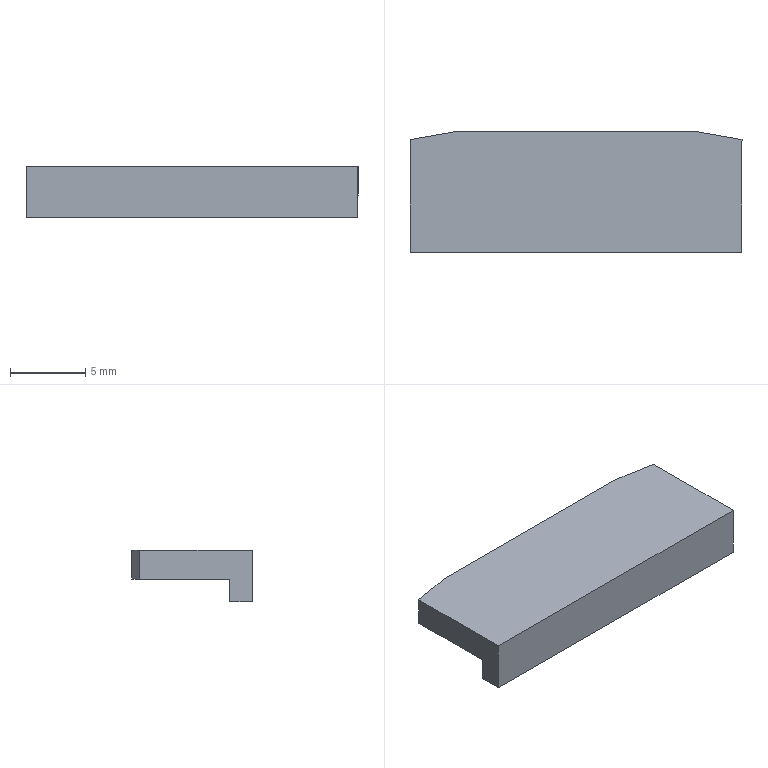Part | NX | 1 solid | 10 faces | box 22 x 8 x 3.4 mm | volume 380.885 mm3 | plane 10
STEP:
#1=CARTESIAN_POINT('',(-35.11,-62.629,7.853));
#2=VERTEX_POINT('',#1);
#3=CARTESIAN_POINT('',(-13.11,-62.629,7.853));
#4=VERTEX_POINT('',#3);
#5=CARTESIAN_POINT('',(-22.513,-62.629,7.853));
#6=DIRECTION('',(1.,0.,0.));
#7=VECTOR('',#6,1000.);
#8=LINE('',#5,#7);
#9=EDGE_CURVE('',#2,#4,#8,.T.);
#10=ORIENTED_EDGE('',*,*,#9,.F.);
#11=CARTESIAN_POINT('',(-35.11,-56.658,7.853));
#12=VERTEX_POINT('',#11);
#13=CARTESIAN_POINT('',(-35.11,-63.129,7.853));
#14=DIRECTION('',(0.,1.,0.));
#15=VECTOR('',#14,1000.);
#16=LINE('',#13,#15);
#17=EDGE_CURVE('',#2,#12,#16,.T.);
#18=ORIENTED_EDGE('',*,*,#17,.T.);
#19=CARTESIAN_POINT('',(-32.11,-56.129,7.853));
#20=VERTEX_POINT('',#19);
#21=CARTESIAN_POINT('',(-22.513,-54.437,7.853));
#22=DIRECTION('',(0.9848,0.1736,0.));
#23=VECTOR('',#22,1000.);
#24=LINE('',#21,#23);
#25=EDGE_CURVE('',#12,#20,#24,.T.);
#26=ORIENTED_EDGE('',*,*,#25,.T.);
#27=CARTESIAN_POINT('',(-16.11,-56.129,7.853));
#28=VERTEX_POINT('',#27);
#29=CARTESIAN_POINT('',(-22.513,-56.129,7.853));
#30=DIRECTION('',(1.,0.,0.));
#31=VECTOR('',#30,1000.);
#32=LINE('',#29,#31);
#33=EDGE_CURVE('',#20,#28,#32,.T.);
#34=ORIENTED_EDGE('',*,*,#33,.T.);
#35=CARTESIAN_POINT('',(-13.11,-56.658,7.853));
#36=VERTEX_POINT('',#35);
#37=CARTESIAN_POINT('',(-22.513,-55.,7.853));
#38=DIRECTION('',(0.9848,-0.1736,0.));
#39=VECTOR('',#38,1000.);
#40=LINE('',#37,#39);
#41=EDGE_CURVE('',#28,#36,#40,.T.);
#42=ORIENTED_EDGE('',*,*,#41,.T.);
#43=CARTESIAN_POINT('',(-13.11,-63.129,7.853));
#44=DIRECTION('',(0.,-1.,0.));
#45=VECTOR('',#44,1000.);
#46=LINE('',#43,#45);
#47=EDGE_CURVE('',#36,#4,#46,.T.);
#48=ORIENTED_EDGE('',*,*,#47,.T.);
#49=EDGE_LOOP('',(#10,#18,#26,#34,#42,#48));
#50=FACE_BOUND('',#49,.T.);
#51=CARTESIAN_POINT('',(-32.11,-63.129,7.853));
#52=DIRECTION('',(0.,0.,-1.));
#53=DIRECTION('',(0.,-1.,0.));
#54=AXIS2_PLACEMENT_3D('',#51,#52,#53);
#55=PLANE('',#54);
#56=ADVANCED_FACE('',(#50),#55,.T.);
#57=CARTESIAN_POINT('',(-35.11,-64.129,6.353));
#58=VERTEX_POINT('',#57);
#59=CARTESIAN_POINT('',(-35.11,-64.129,9.753));
#60=VERTEX_POINT('',#59);
#61=CARTESIAN_POINT('',(-35.11,-64.129,13.966));
#62=DIRECTION('',(0.,0.,1.));
#63=VECTOR('',#62,1000.);
#64=LINE('',#61,#63);
#65=EDGE_CURVE('',#58,#60,#64,.T.);
#66=ORIENTED_EDGE('',*,*,#65,.T.);
#67=CARTESIAN_POINT('',(-35.11,-56.658,9.753));
#68=VERTEX_POINT('',#67);
#69=CARTESIAN_POINT('',(-35.11,-63.129,9.753));
#70=DIRECTION('',(0.,1.,0.));
#71=VECTOR('',#70,1000.);
#72=LINE('',#69,#71);
#73=EDGE_CURVE('',#60,#68,#72,.T.);
#74=ORIENTED_EDGE('',*,*,#73,.T.);
#75=CARTESIAN_POINT('',(-35.11,-56.658,13.966));
#76=DIRECTION('',(0.,0.,-1.));
#77=VECTOR('',#76,1000.);
#78=LINE('',#75,#77);
#79=EDGE_CURVE('',#68,#12,#78,.T.);
#80=ORIENTED_EDGE('',*,*,#79,.T.);
#81=ORIENTED_EDGE('',*,*,#17,.F.);
#82=CARTESIAN_POINT('',(-35.11,-62.629,6.353));
#83=VERTEX_POINT('',#82);
#84=CARTESIAN_POINT('',(-35.11,-62.629,13.966));
#85=DIRECTION('',(0.,0.,1.));
#86=VECTOR('',#85,1000.);
#87=LINE('',#84,#86);
#88=EDGE_CURVE('',#83,#2,#87,.T.);
#89=ORIENTED_EDGE('',*,*,#88,.F.);
#90=CARTESIAN_POINT('',(-35.11,-63.129,6.353));
#91=DIRECTION('',(0.,1.,0.));
#92=VECTOR('',#91,1000.);
#93=LINE('',#90,#92);
#94=EDGE_CURVE('',#58,#83,#93,.T.);
#95=ORIENTED_EDGE('',*,*,#94,.F.);
#96=EDGE_LOOP('',(#66,#74,#80,#81,#89,#95));
#97=FACE_BOUND('',#96,.T.);
#98=CARTESIAN_POINT('',(-35.11,-63.129,9.253));
#99=DIRECTION('',(-1.,0.,0.));
#100=DIRECTION('',(0.,0.,1.));
#101=AXIS2_PLACEMENT_3D('',#98,#99,#100);
#102=PLANE('',#101);
#103=ADVANCED_FACE('',(#97),#102,.T.);
#104=CARTESIAN_POINT('',(-13.11,-64.129,9.753));
#105=VERTEX_POINT('',#104);
#106=CARTESIAN_POINT('',(-22.513,-64.129,9.753));
#107=DIRECTION('',(-1.,0.,0.));
#108=VECTOR('',#107,1000.);
#109=LINE('',#106,#108);
#110=EDGE_CURVE('',#105,#60,#109,.T.);
#111=ORIENTED_EDGE('',*,*,#110,.F.);
#112=CARTESIAN_POINT('',(-13.11,-56.658,9.753));
#113=VERTEX_POINT('',#112);
#114=CARTESIAN_POINT('',(-13.11,-63.129,9.753));
#115=DIRECTION('',(0.,-1.,0.));
#116=VECTOR('',#115,1000.);
#117=LINE('',#114,#116);
#118=EDGE_CURVE('',#113,#105,#117,.T.);
#119=ORIENTED_EDGE('',*,*,#118,.F.);
#120=CARTESIAN_POINT('',(-16.11,-56.129,9.753));
#121=VERTEX_POINT('',#120);
#122=CARTESIAN_POINT('',(-22.513,-55.,9.753));
#123=DIRECTION('',(-0.9848,0.1736,0.));
#124=VECTOR('',#123,1000.);
#125=LINE('',#122,#124);
#126=EDGE_CURVE('',#113,#121,#125,.T.);
#127=ORIENTED_EDGE('',*,*,#126,.T.);
#128=CARTESIAN_POINT('',(-32.11,-56.129,9.753));
#129=VERTEX_POINT('',#128);
#130=CARTESIAN_POINT('',(-22.513,-56.129,9.753));
#131=DIRECTION('',(-1.,0.,0.));
#132=VECTOR('',#131,1000.);
#133=LINE('',#130,#132);
#134=EDGE_CURVE('',#121,#129,#133,.T.);
#135=ORIENTED_EDGE('',*,*,#134,.T.);
#136=CARTESIAN_POINT('',(-22.513,-54.437,9.753));
#137=DIRECTION('',(-0.9848,-0.1736,0.));
#138=VECTOR('',#137,1000.);
#139=LINE('',#136,#138);
#140=EDGE_CURVE('',#129,#68,#139,.T.);
#141=ORIENTED_EDGE('',*,*,#140,.T.);
#142=ORIENTED_EDGE('',*,*,#73,.F.);
#143=EDGE_LOOP('',(#111,#119,#127,#135,#141,#142));
#144=FACE_BOUND('',#143,.T.);
#145=CARTESIAN_POINT('',(-16.11,-63.129,9.753));
#146=DIRECTION('',(0.,0.,1.));
#147=DIRECTION('',(1.,0.,0.));
#148=AXIS2_PLACEMENT_3D('',#145,#146,#147);
#149=PLANE('',#148);
#150=ADVANCED_FACE('',(#144),#149,.T.);
#151=CARTESIAN_POINT('',(-13.11,-64.129,6.353));
#152=VERTEX_POINT('',#151);
#153=CARTESIAN_POINT('',(-13.11,-64.129,13.966));
#154=DIRECTION('',(0.,0.,-1.));
#155=VECTOR('',#154,1000.);
#156=LINE('',#153,#155);
#157=EDGE_CURVE('',#105,#152,#156,.T.);
#158=ORIENTED_EDGE('',*,*,#157,.T.);
#159=CARTESIAN_POINT('',(-13.11,-62.629,6.353));
#160=VERTEX_POINT('',#159);
#161=CARTESIAN_POINT('',(-13.11,-63.129,6.353));
#162=DIRECTION('',(0.,-1.,0.));
#163=VECTOR('',#162,1000.);
#164=LINE('',#161,#163);
#165=EDGE_CURVE('',#160,#152,#164,.T.);
#166=ORIENTED_EDGE('',*,*,#165,.F.);
#167=CARTESIAN_POINT('',(-13.11,-62.629,13.966));
#168=DIRECTION('',(0.,0.,-1.));
#169=VECTOR('',#168,1000.);
#170=LINE('',#167,#169);
#171=EDGE_CURVE('',#4,#160,#170,.T.);
#172=ORIENTED_EDGE('',*,*,#171,.F.);
#173=ORIENTED_EDGE('',*,*,#47,.F.);
#174=CARTESIAN_POINT('',(-13.11,-56.658,13.966));
#175=DIRECTION('',(0.,0.,1.));
#176=VECTOR('',#175,1000.);
#177=LINE('',#174,#176);
#178=EDGE_CURVE('',#36,#113,#177,.T.);
#179=ORIENTED_EDGE('',*,*,#178,.T.);
#180=ORIENTED_EDGE('',*,*,#118,.T.);
#181=EDGE_LOOP('',(#158,#166,#172,#173,#179,#180));
#182=FACE_BOUND('',#181,.T.);
#183=CARTESIAN_POINT('',(-13.11,-63.129,7.853));
#184=DIRECTION('',(1.,0.,0.));
#185=DIRECTION('',(0.,-1.,0.));
#186=AXIS2_PLACEMENT_3D('',#183,#184,#185);
#187=PLANE('',#186);
#188=ADVANCED_FACE('',(#182),#187,.T.);
#189=ORIENTED_EDGE('',*,*,#165,.T.);
#190=CARTESIAN_POINT('',(-22.513,-64.129,6.353));
#191=DIRECTION('',(-1.,0.,0.));
#192=VECTOR('',#191,1000.);
#193=LINE('',#190,#192);
#194=EDGE_CURVE('',#152,#58,#193,.T.);
#195=ORIENTED_EDGE('',*,*,#194,.T.);
#196=ORIENTED_EDGE('',*,*,#94,.T.);
#197=CARTESIAN_POINT('',(-22.513,-62.629,6.353));
#198=DIRECTION('',(1.,0.,0.));
#199=VECTOR('',#198,1000.);
#200=LINE('',#197,#199);
#201=EDGE_CURVE('',#83,#160,#200,.T.);
#202=ORIENTED_EDGE('',*,*,#201,.T.);
#203=EDGE_LOOP('',(#189,#195,#196,#202));
#204=FACE_BOUND('',#203,.T.);
#205=CARTESIAN_POINT('',(-19.282,-63.809,6.353));
#206=DIRECTION('',(0.,0.,-1.));
#207=DIRECTION('',(0.,-1.,0.));
#208=AXIS2_PLACEMENT_3D('',#205,#206,#207);
#209=PLANE('',#208);
#210=ADVANCED_FACE('',(#204),#209,.T.);
#211=CARTESIAN_POINT('',(-32.11,-56.129,13.966));
#212=DIRECTION('',(0.,0.,-1.));
#213=VECTOR('',#212,1000.);
#214=LINE('',#211,#213);
#215=EDGE_CURVE('',#129,#20,#214,.T.);
#216=ORIENTED_EDGE('',*,*,#215,.F.);
#217=ORIENTED_EDGE('',*,*,#134,.F.);
#218=CARTESIAN_POINT('',(-16.11,-56.129,13.966));
#219=DIRECTION('',(0.,0.,1.));
#220=VECTOR('',#219,1000.);
#221=LINE('',#218,#220);
#222=EDGE_CURVE('',#28,#121,#221,.T.);
#223=ORIENTED_EDGE('',*,*,#222,.F.);
#224=ORIENTED_EDGE('',*,*,#33,.F.);
#225=EDGE_LOOP('',(#216,#217,#223,#224));
#226=FACE_BOUND('',#225,.T.);
#227=CARTESIAN_POINT('',(-22.513,-56.129,13.966));
#228=DIRECTION('',(0.,-1.,0.));
#229=DIRECTION('',(-1.,0.,0.));
#230=AXIS2_PLACEMENT_3D('',#227,#228,#229);
#231=PLANE('',#230);
#232=ADVANCED_FACE('',(#226),#231,.F.);
#233=ORIENTED_EDGE('',*,*,#222,.T.);
#234=ORIENTED_EDGE('',*,*,#126,.F.);
#235=ORIENTED_EDGE('',*,*,#178,.F.);
#236=ORIENTED_EDGE('',*,*,#41,.F.);
#237=EDGE_LOOP('',(#233,#234,#235,#236));
#238=FACE_BOUND('',#237,.T.);
#239=CARTESIAN_POINT('',(-14.61,-56.393,8.553));
#240=DIRECTION('',(-0.1736,-0.9848,0.));
#241=DIRECTION('',(-0.9848,0.1736,0.));
#242=AXIS2_PLACEMENT_3D('',#239,#240,#241);
#243=PLANE('',#242);
#244=ADVANCED_FACE('',(#238),#243,.F.);
#245=ORIENTED_EDGE('',*,*,#215,.T.);
#246=ORIENTED_EDGE('',*,*,#25,.F.);
#247=ORIENTED_EDGE('',*,*,#79,.F.);
#248=ORIENTED_EDGE('',*,*,#140,.F.);
#249=EDGE_LOOP('',(#245,#246,#247,#248));
#250=FACE_BOUND('',#249,.T.);
#251=CARTESIAN_POINT('',(-33.61,-56.393,8.553));
#252=DIRECTION('',(0.1736,-0.9848,0.));
#253=DIRECTION('',(0.,0.,-1.));
#254=AXIS2_PLACEMENT_3D('',#251,#252,#253);
#255=PLANE('',#254);
#256=ADVANCED_FACE('',(#250),#255,.F.);
#257=ORIENTED_EDGE('',*,*,#65,.F.);
#258=ORIENTED_EDGE('',*,*,#194,.F.);
#259=ORIENTED_EDGE('',*,*,#157,.F.);
#260=ORIENTED_EDGE('',*,*,#110,.T.);
#261=EDGE_LOOP('',(#257,#258,#259,#260));
#262=FACE_BOUND('',#261,.T.);
#263=CARTESIAN_POINT('',(-22.513,-64.129,13.966));
#264=DIRECTION('',(0.,-1.,0.));
#265=DIRECTION('',(-1.,0.,0.));
#266=AXIS2_PLACEMENT_3D('',#263,#264,#265);
#267=PLANE('',#266);
#268=ADVANCED_FACE('',(#262),#267,.T.);
#269=ORIENTED_EDGE('',*,*,#9,.T.);
#270=ORIENTED_EDGE('',*,*,#171,.T.);
#271=ORIENTED_EDGE('',*,*,#201,.F.);
#272=ORIENTED_EDGE('',*,*,#88,.T.);
#273=EDGE_LOOP('',(#269,#270,#271,#272));
#274=FACE_BOUND('',#273,.T.);
#275=CARTESIAN_POINT('',(-16.21,-62.629,7.853));
#276=DIRECTION('',(0.,1.,0.));
#277=DIRECTION('',(1.,0.,0.));
#278=AXIS2_PLACEMENT_3D('',#275,#276,#277);
#279=PLANE('',#278);
#280=ADVANCED_FACE('',(#274),#279,.T.);
#281=CLOSED_SHELL('',(#56,#103,#150,#188,#210,#232,#244,#256,#268,#280));
#282=MANIFOLD_SOLID_BREP('',#281);
#283=(LENGTH_UNIT()NAMED_UNIT(*)SI_UNIT(.MILLI.,.METRE.));
#284=UNCERTAINTY_MEASURE_WITH_UNIT(LENGTH_MEASURE(0.00001),#283,'','');
#285=(NAMED_UNIT(*)PLANE_ANGLE_UNIT()SI_UNIT($,.RADIAN.));
#286=(NAMED_UNIT(*)SI_UNIT($,.STERADIAN.)SOLID_ANGLE_UNIT());
#287=(GEOMETRIC_REPRESENTATION_CONTEXT(3)GLOBAL_UNCERTAINTY_ASSIGNED_CONTEXT((#284))GLOBAL_UNIT_ASSIGNED_CONTEXT((#283,#285,#286))REPRESENTATION_CONTEXT('',''));
#288=ADVANCED_BREP_SHAPE_REPRESENTATION('',(#282),#287);